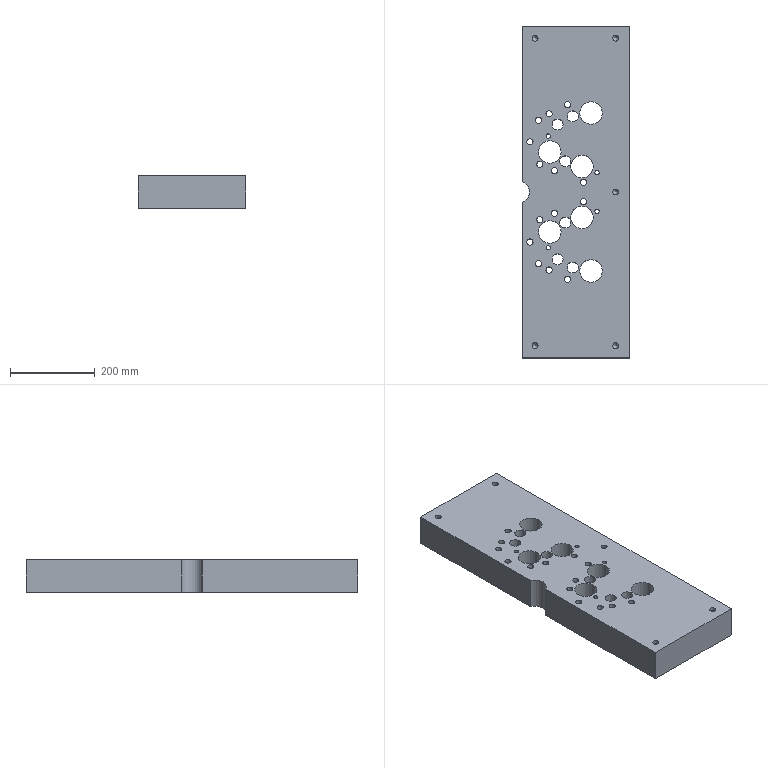Part | NX | features 3 2 | 1 solid | 52 faces | box 253 x 782.437 x 75.5 mm | volume 13452041 mm3 | cylinder 38 | plane 7 | cone 7 | commonest cylinder face diameters 14.5 x14 14.1 x7 53 x7 26 x6 10 x4
STEP:
#1=CARTESIAN_POINT('',(2107.05,-362.5,256.5));
#2=VERTEX_POINT('',#1);
#3=CARTESIAN_POINT('',(2100.,-362.5,256.5));
#4=DIRECTION('',(0.,0.,-1.));
#5=DIRECTION('',(1.,0.,0.));
#6=AXIS2_PLACEMENT_3D('',#3,#4,#5);
#7=CIRCLE('',#6,7.05);
#8=EDGE_CURVE('',#2,#2,#7,.T.);
#9=ORIENTED_EDGE('',*,*,#8,.T.);
#10=EDGE_LOOP('',(#9));
#11=FACE_BOUND('',#10,.T.);
#12=CARTESIAN_POINT('',(1917.05,362.5,256.5));
#13=VERTEX_POINT('',#12);
#14=CARTESIAN_POINT('',(1910.,362.5,256.5));
#15=DIRECTION('',(0.,0.,-1.));
#16=DIRECTION('',(1.,0.,0.));
#17=AXIS2_PLACEMENT_3D('',#14,#15,#16);
#18=CIRCLE('',#17,7.05);
#19=EDGE_CURVE('',#13,#13,#18,.T.);
#20=ORIENTED_EDGE('',*,*,#19,.T.);
#21=EDGE_LOOP('',(#20));
#22=FACE_BOUND('',#21,.T.);
#23=CARTESIAN_POINT('',(2031.25,23.,256.5));
#24=VERTEX_POINT('',#23);
#25=CARTESIAN_POINT('',(2024.,23.,256.5));
#26=DIRECTION('',(0.,0.,-1.));
#27=DIRECTION('',(1.,0.,0.));
#28=AXIS2_PLACEMENT_3D('',#25,#26,#27);
#29=CIRCLE('',#28,7.25);
#30=EDGE_CURVE('',#24,#24,#29,.T.);
#31=ORIENTED_EDGE('',*,*,#30,.T.);
#32=EDGE_LOOP('',(#31));
#33=FACE_BOUND('',#32,.T.);
#34=CARTESIAN_POINT('',(1963.25,50.,256.5));
#35=VERTEX_POINT('',#34);
#36=CARTESIAN_POINT('',(1956.,50.,256.5));
#37=DIRECTION('',(0.,0.,1.));
#38=DIRECTION('',(1.,0.,0.));
#39=AXIS2_PLACEMENT_3D('',#36,#37,#38);
#40=CIRCLE('',#39,7.25);
#41=EDGE_CURVE('',#35,#35,#40,.T.);
#42=ORIENTED_EDGE('',*,*,#41,.F.);
#43=EDGE_LOOP('',(#42));
#44=FACE_BOUND('',#43,.T.);
#45=CARTESIAN_POINT('',(1928.25,65.,256.5));
#46=VERTEX_POINT('',#45);
#47=CARTESIAN_POINT('',(1921.,65.,256.5));
#48=DIRECTION('',(0.,0.,-1.));
#49=DIRECTION('',(1.,0.,0.));
#50=AXIS2_PLACEMENT_3D('',#47,#48,#49);
#51=CIRCLE('',#50,7.25);
#52=EDGE_CURVE('',#46,#46,#51,.T.);
#53=ORIENTED_EDGE('',*,*,#52,.T.);
#54=EDGE_LOOP('',(#53));
#55=FACE_BOUND('',#54,.T.);
#56=CARTESIAN_POINT('',(1905.25,118.,256.5));
#57=VERTEX_POINT('',#56);
#58=CARTESIAN_POINT('',(1898.,118.,256.5));
#59=DIRECTION('',(0.,0.,-1.));
#60=DIRECTION('',(1.,0.,0.));
#61=AXIS2_PLACEMENT_3D('',#58,#59,#60);
#62=CIRCLE('',#61,7.25);
#63=EDGE_CURVE('',#57,#57,#62,.T.);
#64=ORIENTED_EDGE('',*,*,#63,.T.);
#65=EDGE_LOOP('',(#64));
#66=FACE_BOUND('',#65,.T.);
#67=CARTESIAN_POINT('',(1925.25,-169.,256.5));
#68=VERTEX_POINT('',#67);
#69=CARTESIAN_POINT('',(1918.,-169.,256.5));
#70=DIRECTION('',(0.,0.,-1.));
#71=DIRECTION('',(1.,0.,0.));
#72=AXIS2_PLACEMENT_3D('',#69,#70,#71);
#73=CIRCLE('',#72,7.25);
#74=EDGE_CURVE('',#68,#68,#73,.T.);
#75=ORIENTED_EDGE('',*,*,#74,.T.);
#76=EDGE_LOOP('',(#75));
#77=FACE_BOUND('',#76,.T.);
#78=CARTESIAN_POINT('',(1950.25,-184.,256.5));
#79=VERTEX_POINT('',#78);
#80=CARTESIAN_POINT('',(1943.,-184.,256.5));
#81=DIRECTION('',(0.,0.,-1.));
#82=DIRECTION('',(1.,0.,0.));
#83=AXIS2_PLACEMENT_3D('',#80,#81,#82);
#84=CIRCLE('',#83,7.25);
#85=EDGE_CURVE('',#79,#79,#84,.T.);
#86=ORIENTED_EDGE('',*,*,#85,.T.);
#87=EDGE_LOOP('',(#86));
#88=FACE_BOUND('',#87,.T.);
#89=CARTESIAN_POINT('',(1993.25,-206.,256.5));
#90=VERTEX_POINT('',#89);
#91=CARTESIAN_POINT('',(1986.,-206.,256.5));
#92=DIRECTION('',(0.,0.,1.));
#93=DIRECTION('',(1.,0.,0.));
#94=AXIS2_PLACEMENT_3D('',#91,#92,#93);
#95=CIRCLE('',#94,7.25);
#96=EDGE_CURVE('',#90,#90,#95,.T.);
#97=ORIENTED_EDGE('',*,*,#96,.F.);
#98=EDGE_LOOP('',(#97));
#99=FACE_BOUND('',#98,.T.);
#100=CARTESIAN_POINT('',(2012.,-178.,256.5));
#101=VERTEX_POINT('',#100);
#102=CARTESIAN_POINT('',(1999.,-178.,256.5));
#103=DIRECTION('',(0.,0.,-1.));
#104=DIRECTION('',(1.,0.,0.));
#105=AXIS2_PLACEMENT_3D('',#102,#103,#104);
#106=CIRCLE('',#105,13.);
#107=EDGE_CURVE('',#101,#101,#106,.T.);
#108=ORIENTED_EDGE('',*,*,#107,.T.);
#109=EDGE_LOOP('',(#108));
#110=FACE_BOUND('',#109,.T.);
#111=CARTESIAN_POINT('',(1994.,72.,256.5));
#112=VERTEX_POINT('',#111);
#113=CARTESIAN_POINT('',(1981.,72.,256.5));
#114=DIRECTION('',(0.,0.,-1.));
#115=DIRECTION('',(1.,0.,0.));
#116=AXIS2_PLACEMENT_3D('',#113,#114,#115);
#117=CIRCLE('',#116,13.);
#118=EDGE_CURVE('',#112,#112,#117,.T.);
#119=ORIENTED_EDGE('',*,*,#118,.T.);
#120=EDGE_LOOP('',(#119));
#121=FACE_BOUND('',#120,.T.);
#122=CARTESIAN_POINT('',(1994.,-72.,256.5));
#123=VERTEX_POINT('',#122);
#124=CARTESIAN_POINT('',(1981.,-72.,256.5));
#125=DIRECTION('',(0.,0.,-1.));
#126=DIRECTION('',(1.,0.,0.));
#127=AXIS2_PLACEMENT_3D('',#124,#125,#126);
#128=CIRCLE('',#127,13.);
#129=EDGE_CURVE('',#123,#123,#128,.T.);
#130=ORIENTED_EDGE('',*,*,#129,.T.);
#131=EDGE_LOOP('',(#130));
#132=FACE_BOUND('',#131,.T.);
#133=CARTESIAN_POINT('',(1976.,159.,256.5));
#134=VERTEX_POINT('',#133);
#135=CARTESIAN_POINT('',(1963.,159.,256.5));
#136=DIRECTION('',(0.,0.,-1.));
#137=DIRECTION('',(1.,0.,0.));
#138=AXIS2_PLACEMENT_3D('',#135,#136,#137);
#139=CIRCLE('',#138,13.);
#140=EDGE_CURVE('',#134,#134,#139,.T.);
#141=ORIENTED_EDGE('',*,*,#140,.T.);
#142=EDGE_LOOP('',(#141));
#143=FACE_BOUND('',#142,.T.);
#144=CARTESIAN_POINT('',(1976.,-159.,256.5));
#145=VERTEX_POINT('',#144);
#146=CARTESIAN_POINT('',(1963.,-159.,256.5));
#147=DIRECTION('',(0.,0.,-1.));
#148=DIRECTION('',(1.,0.,0.));
#149=AXIS2_PLACEMENT_3D('',#146,#147,#148);
#150=CIRCLE('',#149,13.);
#151=EDGE_CURVE('',#145,#145,#150,.T.);
#152=ORIENTED_EDGE('',*,*,#151,.T.);
#153=EDGE_LOOP('',(#152));
#154=FACE_BOUND('',#153,.T.);
#155=CARTESIAN_POINT('',(1945.861,131.692,256.5));
#156=VERTEX_POINT('',#155);
#157=CARTESIAN_POINT('',(1940.861,131.692,256.5));
#158=DIRECTION('',(0.,0.,-1.));
#159=DIRECTION('',(1.,0.,0.));
#160=AXIS2_PLACEMENT_3D('',#157,#158,#159);
#161=CIRCLE('',#160,5.);
#162=EDGE_CURVE('',#156,#156,#161,.T.);
#163=ORIENTED_EDGE('',*,*,#162,.T.);
#164=EDGE_LOOP('',(#163));
#165=FACE_BOUND('',#164,.T.);
#166=CARTESIAN_POINT('',(2012.,178.,256.5));
#167=VERTEX_POINT('',#166);
#168=CARTESIAN_POINT('',(1999.,178.,256.5));
#169=DIRECTION('',(0.,0.,-1.));
#170=DIRECTION('',(1.,0.,0.));
#171=AXIS2_PLACEMENT_3D('',#168,#169,#170);
#172=CIRCLE('',#171,13.);
#173=EDGE_CURVE('',#167,#167,#172,.T.);
#174=ORIENTED_EDGE('',*,*,#173,.T.);
#175=EDGE_LOOP('',(#174));
#176=FACE_BOUND('',#175,.T.);
#177=CARTESIAN_POINT('',(2060.861,-45.692,256.5));
#178=VERTEX_POINT('',#177);
#179=CARTESIAN_POINT('',(2055.861,-45.692,256.5));
#180=DIRECTION('',(0.,0.,-1.));
#181=DIRECTION('',(1.,0.,0.));
#182=AXIS2_PLACEMENT_3D('',#179,#180,#181);
#183=CIRCLE('',#182,5.);
#184=EDGE_CURVE('',#178,#178,#183,.T.);
#185=ORIENTED_EDGE('',*,*,#184,.T.);
#186=EDGE_LOOP('',(#185));
#187=FACE_BOUND('',#186,.T.);
#188=CARTESIAN_POINT('',(2060.861,45.692,256.5));
#189=VERTEX_POINT('',#188);
#190=CARTESIAN_POINT('',(2055.861,45.692,256.5));
#191=DIRECTION('',(0.,0.,-1.));
#192=DIRECTION('',(1.,0.,0.));
#193=AXIS2_PLACEMENT_3D('',#190,#191,#192);
#194=CIRCLE('',#193,5.);
#195=EDGE_CURVE('',#189,#189,#194,.T.);
#196=ORIENTED_EDGE('',*,*,#195,.T.);
#197=EDGE_LOOP('',(#196));
#198=FACE_BOUND('',#197,.T.);
#199=CARTESIAN_POINT('',(2047.195,60.048,256.5));
#200=VERTEX_POINT('',#199);
#201=CARTESIAN_POINT('',(2020.695,60.048,256.5));
#202=DIRECTION('',(0.,0.,-1.));
#203=DIRECTION('',(1.,0.,0.));
#204=AXIS2_PLACEMENT_3D('',#201,#202,#203);
#205=CIRCLE('',#204,26.5);
#206=EDGE_CURVE('',#200,#200,#205,.T.);
#207=ORIENTED_EDGE('',*,*,#206,.T.);
#208=EDGE_LOOP('',(#207));
#209=FACE_BOUND('',#208,.T.);
#210=CARTESIAN_POINT('',(2047.195,-60.048,256.5));
#211=VERTEX_POINT('',#210);
#212=CARTESIAN_POINT('',(2020.695,-60.048,256.5));
#213=DIRECTION('',(0.,0.,-1.));
#214=DIRECTION('',(1.,0.,0.));
#215=AXIS2_PLACEMENT_3D('',#212,#213,#214);
#216=CIRCLE('',#215,26.5);
#217=EDGE_CURVE('',#211,#211,#216,.T.);
#218=ORIENTED_EDGE('',*,*,#217,.T.);
#219=EDGE_LOOP('',(#218));
#220=FACE_BOUND('',#219,.T.);
#221=CARTESIAN_POINT('',(2068.5,-186.,256.5));
#222=VERTEX_POINT('',#221);
#223=CARTESIAN_POINT('',(2042.,-186.,256.5));
#224=DIRECTION('',(0.,0.,-1.));
#225=DIRECTION('',(1.,0.,0.));
#226=AXIS2_PLACEMENT_3D('',#223,#224,#225);
#227=CIRCLE('',#226,26.5);
#228=EDGE_CURVE('',#222,#222,#227,.T.);
#229=ORIENTED_EDGE('',*,*,#228,.T.);
#230=EDGE_LOOP('',(#229));
#231=FACE_BOUND('',#230,.T.);
#232=CARTESIAN_POINT('',(1971.5,94.,256.5));
#233=VERTEX_POINT('',#232);
#234=CARTESIAN_POINT('',(1945.,94.,256.5));
#235=DIRECTION('',(0.,0.,1.));
#236=DIRECTION('',(1.,0.,0.));
#237=AXIS2_PLACEMENT_3D('',#234,#235,#236);
#238=CIRCLE('',#237,26.5);
#239=EDGE_CURVE('',#233,#233,#238,.T.);
#240=ORIENTED_EDGE('',*,*,#239,.F.);
#241=EDGE_LOOP('',(#240));
#242=FACE_BOUND('',#241,.T.);
#243=CARTESIAN_POINT('',(1880.,-24.541,256.5));
#244=VERTEX_POINT('',#243);
#245=CARTESIAN_POINT('',(1880.,24.541,256.5));
#246=VERTEX_POINT('',#245);
#247=CARTESIAN_POINT('',(1870.,0.,256.5));
#248=DIRECTION('',(0.,0.,1.));
#249=DIRECTION('',(1.,0.,0.));
#250=AXIS2_PLACEMENT_3D('',#247,#248,#249);
#251=CIRCLE('',#250,26.5);
#252=EDGE_CURVE('',#244,#246,#251,.T.);
#253=ORIENTED_EDGE('',*,*,#252,.F.);
#254=CARTESIAN_POINT('',(1880.,-391.218,256.5));
#255=VERTEX_POINT('',#254);
#256=CARTESIAN_POINT('',(1880.,193.,256.5));
#257=DIRECTION('',(0.,1.,0.));
#258=VECTOR('',#257,1000.);
#259=LINE('',#256,#258);
#260=EDGE_CURVE('',#255,#244,#259,.T.);
#261=ORIENTED_EDGE('',*,*,#260,.F.);
#262=CARTESIAN_POINT('',(2133.,-391.218,256.5));
#263=VERTEX_POINT('',#262);
#264=CARTESIAN_POINT('',(4065.,-391.218,256.5));
#265=DIRECTION('',(1.,0.,0.));
#266=VECTOR('',#265,1000.);
#267=LINE('',#264,#266);
#268=EDGE_CURVE('',#255,#263,#267,.T.);
#269=ORIENTED_EDGE('',*,*,#268,.T.);
#270=CARTESIAN_POINT('',(2133.,391.218,256.5));
#271=VERTEX_POINT('',#270);
#272=CARTESIAN_POINT('',(2133.,193.,256.5));
#273=DIRECTION('',(0.,-1.,0.));
#274=VECTOR('',#273,1000.);
#275=LINE('',#272,#274);
#276=EDGE_CURVE('',#271,#263,#275,.T.);
#277=ORIENTED_EDGE('',*,*,#276,.F.);
#278=CARTESIAN_POINT('',(1880.,391.218,256.5));
#279=VERTEX_POINT('',#278);
#280=CARTESIAN_POINT('',(4065.,391.218,256.5));
#281=DIRECTION('',(1.,0.,0.));
#282=VECTOR('',#281,1000.);
#283=LINE('',#280,#282);
#284=EDGE_CURVE('',#279,#271,#283,.T.);
#285=ORIENTED_EDGE('',*,*,#284,.F.);
#286=CARTESIAN_POINT('',(1880.,193.,256.5));
#287=DIRECTION('',(0.,1.,0.));
#288=VECTOR('',#287,1000.);
#289=LINE('',#286,#288);
#290=EDGE_CURVE('',#246,#279,#289,.T.);
#291=ORIENTED_EDGE('',*,*,#290,.F.);
#292=EDGE_LOOP('',(#253,#261,#269,#277,#285,#291));
#293=FACE_BOUND('',#292,.T.);
#294=CARTESIAN_POINT('',(1971.5,-94.,256.5));
#295=VERTEX_POINT('',#294);
#296=CARTESIAN_POINT('',(1945.,-94.,256.5));
#297=DIRECTION('',(0.,0.,-1.));
#298=DIRECTION('',(1.,0.,0.));
#299=AXIS2_PLACEMENT_3D('',#296,#297,#298);
#300=CIRCLE('',#299,26.5);
#301=EDGE_CURVE('',#295,#295,#300,.T.);
#302=ORIENTED_EDGE('',*,*,#301,.T.);
#303=EDGE_LOOP('',(#302));
#304=FACE_BOUND('',#303,.T.);
#305=CARTESIAN_POINT('',(2068.5,186.,256.5));
#306=VERTEX_POINT('',#305);
#307=CARTESIAN_POINT('',(2042.,186.,256.5));
#308=DIRECTION('',(0.,0.,1.));
#309=DIRECTION('',(1.,0.,0.));
#310=AXIS2_PLACEMENT_3D('',#307,#308,#309);
#311=CIRCLE('',#310,26.5);
#312=EDGE_CURVE('',#306,#306,#311,.T.);
#313=ORIENTED_EDGE('',*,*,#312,.F.);
#314=EDGE_LOOP('',(#313));
#315=FACE_BOUND('',#314,.T.);
#316=CARTESIAN_POINT('',(1945.861,-131.692,256.5));
#317=VERTEX_POINT('',#316);
#318=CARTESIAN_POINT('',(1940.861,-131.692,256.5));
#319=DIRECTION('',(0.,0.,-1.));
#320=DIRECTION('',(1.,0.,0.));
#321=AXIS2_PLACEMENT_3D('',#318,#319,#320);
#322=CIRCLE('',#321,5.);
#323=EDGE_CURVE('',#317,#317,#322,.T.);
#324=ORIENTED_EDGE('',*,*,#323,.T.);
#325=EDGE_LOOP('',(#324));
#326=FACE_BOUND('',#325,.T.);
#327=CARTESIAN_POINT('',(2031.25,-23.,256.5));
#328=VERTEX_POINT('',#327);
#329=CARTESIAN_POINT('',(2024.,-23.,256.5));
#330=DIRECTION('',(0.,0.,-1.));
#331=DIRECTION('',(1.,0.,0.));
#332=AXIS2_PLACEMENT_3D('',#329,#330,#331);
#333=CIRCLE('',#332,7.25);
#334=EDGE_CURVE('',#328,#328,#333,.T.);
#335=ORIENTED_EDGE('',*,*,#334,.T.);
#336=EDGE_LOOP('',(#335));
#337=FACE_BOUND('',#336,.T.);
#338=CARTESIAN_POINT('',(1963.25,-50.,256.5));
#339=VERTEX_POINT('',#338);
#340=CARTESIAN_POINT('',(1956.,-50.,256.5));
#341=DIRECTION('',(0.,0.,-1.));
#342=DIRECTION('',(1.,0.,0.));
#343=AXIS2_PLACEMENT_3D('',#340,#341,#342);
#344=CIRCLE('',#343,7.25);
#345=EDGE_CURVE('',#339,#339,#344,.T.);
#346=ORIENTED_EDGE('',*,*,#345,.T.);
#347=EDGE_LOOP('',(#346));
#348=FACE_BOUND('',#347,.T.);
#349=CARTESIAN_POINT('',(1928.25,-65.,256.5));
#350=VERTEX_POINT('',#349);
#351=CARTESIAN_POINT('',(1921.,-65.,256.5));
#352=DIRECTION('',(0.,0.,1.));
#353=DIRECTION('',(1.,0.,0.));
#354=AXIS2_PLACEMENT_3D('',#351,#352,#353);
#355=CIRCLE('',#354,7.25);
#356=EDGE_CURVE('',#350,#350,#355,.T.);
#357=ORIENTED_EDGE('',*,*,#356,.F.);
#358=EDGE_LOOP('',(#357));
#359=FACE_BOUND('',#358,.T.);
#360=CARTESIAN_POINT('',(1905.25,-118.,256.5));
#361=VERTEX_POINT('',#360);
#362=CARTESIAN_POINT('',(1898.,-118.,256.5));
#363=DIRECTION('',(0.,0.,-1.));
#364=DIRECTION('',(1.,0.,0.));
#365=AXIS2_PLACEMENT_3D('',#362,#363,#364);
#366=CIRCLE('',#365,7.25);
#367=EDGE_CURVE('',#361,#361,#366,.T.);
#368=ORIENTED_EDGE('',*,*,#367,.T.);
#369=EDGE_LOOP('',(#368));
#370=FACE_BOUND('',#369,.T.);
#371=CARTESIAN_POINT('',(1925.25,169.,256.5));
#372=VERTEX_POINT('',#371);
#373=CARTESIAN_POINT('',(1918.,169.,256.5));
#374=DIRECTION('',(0.,0.,-1.));
#375=DIRECTION('',(1.,0.,0.));
#376=AXIS2_PLACEMENT_3D('',#373,#374,#375);
#377=CIRCLE('',#376,7.25);
#378=EDGE_CURVE('',#372,#372,#377,.T.);
#379=ORIENTED_EDGE('',*,*,#378,.T.);
#380=EDGE_LOOP('',(#379));
#381=FACE_BOUND('',#380,.T.);
#382=CARTESIAN_POINT('',(1950.25,184.,256.5));
#383=VERTEX_POINT('',#382);
#384=CARTESIAN_POINT('',(1943.,184.,256.5));
#385=DIRECTION('',(0.,0.,-1.));
#386=DIRECTION('',(1.,0.,0.));
#387=AXIS2_PLACEMENT_3D('',#384,#385,#386);
#388=CIRCLE('',#387,7.25);
#389=EDGE_CURVE('',#383,#383,#388,.T.);
#390=ORIENTED_EDGE('',*,*,#389,.T.);
#391=EDGE_LOOP('',(#390));
#392=FACE_BOUND('',#391,.T.);
#393=CARTESIAN_POINT('',(1993.25,206.,256.5));
#394=VERTEX_POINT('',#393);
#395=CARTESIAN_POINT('',(1986.,206.,256.5));
#396=DIRECTION('',(0.,0.,-1.));
#397=DIRECTION('',(1.,0.,0.));
#398=AXIS2_PLACEMENT_3D('',#395,#396,#397);
#399=CIRCLE('',#398,7.25);
#400=EDGE_CURVE('',#394,#394,#399,.T.);
#401=ORIENTED_EDGE('',*,*,#400,.T.);
#402=EDGE_LOOP('',(#401));
#403=FACE_BOUND('',#402,.T.);
#404=CARTESIAN_POINT('',(1917.05,-362.5,256.5));
#405=VERTEX_POINT('',#404);
#406=CARTESIAN_POINT('',(1910.,-362.5,256.5));
#407=DIRECTION('',(0.,0.,-1.));
#408=DIRECTION('',(1.,0.,0.));
#409=AXIS2_PLACEMENT_3D('',#406,#407,#408);
#410=CIRCLE('',#409,7.05);
#411=EDGE_CURVE('',#405,#405,#410,.T.);
#412=ORIENTED_EDGE('',*,*,#411,.T.);
#413=EDGE_LOOP('',(#412));
#414=FACE_BOUND('',#413,.T.);
#415=CARTESIAN_POINT('',(2107.05,362.5,256.5));
#416=VERTEX_POINT('',#415);
#417=CARTESIAN_POINT('',(2100.,362.5,256.5));
#418=DIRECTION('',(0.,0.,-1.));
#419=DIRECTION('',(1.,0.,0.));
#420=AXIS2_PLACEMENT_3D('',#417,#418,#419);
#421=CIRCLE('',#420,7.05);
#422=EDGE_CURVE('',#416,#416,#421,.T.);
#423=ORIENTED_EDGE('',*,*,#422,.T.);
#424=EDGE_LOOP('',(#423));
#425=FACE_BOUND('',#424,.T.);
#426=CARTESIAN_POINT('',(2107.05,0.,256.5));
#427=VERTEX_POINT('',#426);
#428=CARTESIAN_POINT('',(2100.,0.,256.5));
#429=DIRECTION('',(0.,0.,-1.));
#430=DIRECTION('',(1.,0.,0.));
#431=AXIS2_PLACEMENT_3D('',#428,#429,#430);
#432=CIRCLE('',#431,7.05);
#433=EDGE_CURVE('',#427,#427,#432,.T.);
#434=ORIENTED_EDGE('',*,*,#433,.T.);
#435=EDGE_LOOP('',(#434));
#436=FACE_BOUND('',#435,.T.);
#437=CARTESIAN_POINT('',(4065.,0.,256.5));
#438=DIRECTION('',(0.,0.,1.));
#439=DIRECTION('',(-1.,0.,0.));
#440=AXIS2_PLACEMENT_3D('',#437,#438,#439);
#441=PLANE('',#440);
#442=ADVANCED_FACE('',(#11,#22,#33,#44,#55,#66,#77,#88,#99,#110,#121,#132,#143,#154,#165,#176,#187,#198,#209,#220,#231,#242,#293,#304,#315,#326,#337,#348,#359,#370,#381,#392,#403,#414,#425,#436),#441,.T.);
#443=CARTESIAN_POINT('',(1935.861,131.692,181.));
#444=VERTEX_POINT('',#443);
#445=CARTESIAN_POINT('',(1940.861,131.692,181.));
#446=DIRECTION('',(0.,0.,-1.));
#447=DIRECTION('',(-1.,0.,0.));
#448=AXIS2_PLACEMENT_3D('',#445,#446,#447);
#449=CIRCLE('',#448,5.);
#450=EDGE_CURVE('',#444,#444,#449,.T.);
#451=ORIENTED_EDGE('',*,*,#450,.F.);
#452=EDGE_LOOP('',(#451));
#453=FACE_BOUND('',#452,.T.);
#454=CARTESIAN_POINT('',(2050.861,45.692,181.));
#455=VERTEX_POINT('',#454);
#456=CARTESIAN_POINT('',(2055.861,45.692,181.));
#457=DIRECTION('',(0.,0.,-1.));
#458=DIRECTION('',(-1.,0.,0.));
#459=AXIS2_PLACEMENT_3D('',#456,#457,#458);
#460=CIRCLE('',#459,5.);
#461=EDGE_CURVE('',#455,#455,#460,.T.);
#462=ORIENTED_EDGE('',*,*,#461,.F.);
#463=EDGE_LOOP('',(#462));
#464=FACE_BOUND('',#463,.T.);
#465=CARTESIAN_POINT('',(2050.861,-45.692,181.));
#466=VERTEX_POINT('',#465);
#467=CARTESIAN_POINT('',(2055.861,-45.692,181.));
#468=DIRECTION('',(0.,0.,-1.));
#469=DIRECTION('',(-1.,0.,0.));
#470=AXIS2_PLACEMENT_3D('',#467,#468,#469);
#471=CIRCLE('',#470,5.);
#472=EDGE_CURVE('',#466,#466,#471,.T.);
#473=ORIENTED_EDGE('',*,*,#472,.F.);
#474=EDGE_LOOP('',(#473));
#475=FACE_BOUND('',#474,.T.);
#476=CARTESIAN_POINT('',(1935.861,-131.692,181.));
#477=VERTEX_POINT('',#476);
#478=CARTESIAN_POINT('',(1940.861,-131.692,181.));
#479=DIRECTION('',(0.,0.,-1.));
#480=DIRECTION('',(-1.,0.,0.));
#481=AXIS2_PLACEMENT_3D('',#478,#479,#480);
#482=CIRCLE('',#481,5.);
#483=EDGE_CURVE('',#477,#477,#482,.T.);
#484=ORIENTED_EDGE('',*,*,#483,.F.);
#485=EDGE_LOOP('',(#484));
#486=FACE_BOUND('',#485,.T.);
#487=CARTESIAN_POINT('',(1917.05,-362.5,181.));
#488=VERTEX_POINT('',#487);
#489=CARTESIAN_POINT('',(1910.,-362.5,181.));
#490=DIRECTION('',(0.,0.,1.));
#491=DIRECTION('',(1.,0.,0.));
#492=AXIS2_PLACEMENT_3D('',#489,#490,#491);
#493=CIRCLE('',#492,7.05);
#494=EDGE_CURVE('',#488,#488,#493,.T.);
#495=ORIENTED_EDGE('',*,*,#494,.T.);
#496=EDGE_LOOP('',(#495));
#497=FACE_BOUND('',#496,.T.);
#498=CARTESIAN_POINT('',(1978.75,206.,181.));
#499=VERTEX_POINT('',#498);
#500=CARTESIAN_POINT('',(1986.,206.,181.));
#501=DIRECTION('',(0.,0.,-1.));
#502=DIRECTION('',(-1.,0.,0.));
#503=AXIS2_PLACEMENT_3D('',#500,#501,#502);
#504=CIRCLE('',#503,7.25);
#505=EDGE_CURVE('',#499,#499,#504,.T.);
#506=ORIENTED_EDGE('',*,*,#505,.F.);
#507=EDGE_LOOP('',(#506));
#508=FACE_BOUND('',#507,.T.);
#509=CARTESIAN_POINT('',(1935.75,184.,181.));
#510=VERTEX_POINT('',#509);
#511=CARTESIAN_POINT('',(1943.,184.,181.));
#512=DIRECTION('',(0.,0.,-1.));
#513=DIRECTION('',(-1.,0.,0.));
#514=AXIS2_PLACEMENT_3D('',#511,#512,#513);
#515=CIRCLE('',#514,7.25);
#516=EDGE_CURVE('',#510,#510,#515,.T.);
#517=ORIENTED_EDGE('',*,*,#516,.F.);
#518=EDGE_LOOP('',(#517));
#519=FACE_BOUND('',#518,.T.);
#520=CARTESIAN_POINT('',(1910.75,169.,181.));
#521=VERTEX_POINT('',#520);
#522=CARTESIAN_POINT('',(1918.,169.,181.));
#523=DIRECTION('',(0.,0.,1.));
#524=DIRECTION('',(-1.,0.,0.));
#525=AXIS2_PLACEMENT_3D('',#522,#523,#524);
#526=CIRCLE('',#525,7.25);
#527=EDGE_CURVE('',#521,#521,#526,.T.);
#528=ORIENTED_EDGE('',*,*,#527,.T.);
#529=EDGE_LOOP('',(#528));
#530=FACE_BOUND('',#529,.T.);
#531=CARTESIAN_POINT('',(1890.75,-118.,181.));
#532=VERTEX_POINT('',#531);
#533=CARTESIAN_POINT('',(1898.,-118.,181.));
#534=DIRECTION('',(0.,0.,1.));
#535=DIRECTION('',(-1.,0.,0.));
#536=AXIS2_PLACEMENT_3D('',#533,#534,#535);
#537=CIRCLE('',#536,7.25);
#538=EDGE_CURVE('',#532,#532,#537,.T.);
#539=ORIENTED_EDGE('',*,*,#538,.T.);
#540=EDGE_LOOP('',(#539));
#541=FACE_BOUND('',#540,.T.);
#542=CARTESIAN_POINT('',(1913.75,-65.,181.));
#543=VERTEX_POINT('',#542);
#544=CARTESIAN_POINT('',(1921.,-65.,181.));
#545=DIRECTION('',(0.,0.,1.));
#546=DIRECTION('',(-1.,0.,0.));
#547=AXIS2_PLACEMENT_3D('',#544,#545,#546);
#548=CIRCLE('',#547,7.25);
#549=EDGE_CURVE('',#543,#543,#548,.T.);
#550=ORIENTED_EDGE('',*,*,#549,.T.);
#551=EDGE_LOOP('',(#550));
#552=FACE_BOUND('',#551,.T.);
#553=CARTESIAN_POINT('',(1948.75,-50.,181.));
#554=VERTEX_POINT('',#553);
#555=CARTESIAN_POINT('',(1956.,-50.,181.));
#556=DIRECTION('',(0.,0.,-1.));
#557=DIRECTION('',(-1.,0.,0.));
#558=AXIS2_PLACEMENT_3D('',#555,#556,#557);
#559=CIRCLE('',#558,7.25);
#560=EDGE_CURVE('',#554,#554,#559,.T.);
#561=ORIENTED_EDGE('',*,*,#560,.F.);
#562=EDGE_LOOP('',(#561));
#563=FACE_BOUND('',#562,.T.);
#564=CARTESIAN_POINT('',(2016.75,-23.,181.));
#565=VERTEX_POINT('',#564);
#566=CARTESIAN_POINT('',(2024.,-23.,181.));
#567=DIRECTION('',(0.,0.,1.));
#568=DIRECTION('',(-1.,0.,0.));
#569=AXIS2_PLACEMENT_3D('',#566,#567,#568);
#570=CIRCLE('',#569,7.25);
#571=EDGE_CURVE('',#565,#565,#570,.T.);
#572=ORIENTED_EDGE('',*,*,#571,.T.);
#573=EDGE_LOOP('',(#572));
#574=FACE_BOUND('',#573,.T.);
#575=CARTESIAN_POINT('',(2015.5,186.,181.));
#576=VERTEX_POINT('',#575);
#577=CARTESIAN_POINT('',(2042.,186.,181.));
#578=DIRECTION('',(0.,0.,1.));
#579=DIRECTION('',(-1.,0.,0.));
#580=AXIS2_PLACEMENT_3D('',#577,#578,#579);
#581=CIRCLE('',#580,26.5);
#582=EDGE_CURVE('',#576,#576,#581,.T.);
#583=ORIENTED_EDGE('',*,*,#582,.T.);
#584=EDGE_LOOP('',(#583));
#585=FACE_BOUND('',#584,.T.);
#586=CARTESIAN_POINT('',(1918.5,-94.,181.));
#587=VERTEX_POINT('',#586);
#588=CARTESIAN_POINT('',(1945.,-94.,181.));
#589=DIRECTION('',(0.,0.,-1.));
#590=DIRECTION('',(-1.,0.,0.));
#591=AXIS2_PLACEMENT_3D('',#588,#589,#590);
#592=CIRCLE('',#591,26.5);
#593=EDGE_CURVE('',#587,#587,#592,.T.);
#594=ORIENTED_EDGE('',*,*,#593,.F.);
#595=EDGE_LOOP('',(#594));
#596=FACE_BOUND('',#595,.T.);
#597=CARTESIAN_POINT('',(1880.,-24.541,181.));
#598=VERTEX_POINT('',#597);
#599=CARTESIAN_POINT('',(1880.,24.541,181.));
#600=VERTEX_POINT('',#599);
#601=CARTESIAN_POINT('',(1870.,0.,181.));
#602=DIRECTION('',(0.,0.,1.));
#603=DIRECTION('',(-1.,0.,0.));
#604=AXIS2_PLACEMENT_3D('',#601,#602,#603);
#605=CIRCLE('',#604,26.5);
#606=EDGE_CURVE('',#598,#600,#605,.T.);
#607=ORIENTED_EDGE('',*,*,#606,.T.);
#608=CARTESIAN_POINT('',(1880.,391.218,181.));
#609=VERTEX_POINT('',#608);
#610=CARTESIAN_POINT('',(1880.,193.,181.));
#611=DIRECTION('',(0.,-1.,0.));
#612=VECTOR('',#611,1000.);
#613=LINE('',#610,#612);
#614=EDGE_CURVE('',#609,#600,#613,.T.);
#615=ORIENTED_EDGE('',*,*,#614,.F.);
#616=CARTESIAN_POINT('',(2133.,391.218,181.));
#617=VERTEX_POINT('',#616);
#618=CARTESIAN_POINT('',(3295.,391.218,181.));
#619=DIRECTION('',(-1.,0.,0.));
#620=VECTOR('',#619,1000.);
#621=LINE('',#618,#620);
#622=EDGE_CURVE('',#617,#609,#621,.T.);
#623=ORIENTED_EDGE('',*,*,#622,.F.);
#624=CARTESIAN_POINT('',(2133.,-391.218,181.));
#625=VERTEX_POINT('',#624);
#626=CARTESIAN_POINT('',(2133.,193.,181.));
#627=DIRECTION('',(0.,1.,0.));
#628=VECTOR('',#627,1000.);
#629=LINE('',#626,#628);
#630=EDGE_CURVE('',#625,#617,#629,.T.);
#631=ORIENTED_EDGE('',*,*,#630,.F.);
#632=CARTESIAN_POINT('',(1880.,-391.218,181.));
#633=VERTEX_POINT('',#632);
#634=CARTESIAN_POINT('',(3295.,-391.218,181.));
#635=DIRECTION('',(-1.,0.,0.));
#636=VECTOR('',#635,1000.);
#637=LINE('',#634,#636);
#638=EDGE_CURVE('',#625,#633,#637,.T.);
#639=ORIENTED_EDGE('',*,*,#638,.T.);
#640=CARTESIAN_POINT('',(1880.,193.,181.));
#641=DIRECTION('',(0.,-1.,0.));
#642=VECTOR('',#641,1000.);
#643=LINE('',#640,#642);
#644=EDGE_CURVE('',#598,#633,#643,.T.);
#645=ORIENTED_EDGE('',*,*,#644,.F.);
#646=EDGE_LOOP('',(#607,#615,#623,#631,#639,#645));
#647=FACE_BOUND('',#646,.T.);
#648=CARTESIAN_POINT('',(1918.5,94.,181.));
#649=VERTEX_POINT('',#648);
#650=CARTESIAN_POINT('',(1945.,94.,181.));
#651=DIRECTION('',(0.,0.,1.));
#652=DIRECTION('',(-1.,0.,0.));
#653=AXIS2_PLACEMENT_3D('',#650,#651,#652);
#654=CIRCLE('',#653,26.5);
#655=EDGE_CURVE('',#649,#649,#654,.T.);
#656=ORIENTED_EDGE('',*,*,#655,.T.);
#657=EDGE_LOOP('',(#656));
#658=FACE_BOUND('',#657,.T.);
#659=CARTESIAN_POINT('',(2015.5,-186.,181.));
#660=VERTEX_POINT('',#659);
#661=CARTESIAN_POINT('',(2042.,-186.,181.));
#662=DIRECTION('',(0.,0.,-1.));
#663=DIRECTION('',(-1.,0.,0.));
#664=AXIS2_PLACEMENT_3D('',#661,#662,#663);
#665=CIRCLE('',#664,26.5);
#666=EDGE_CURVE('',#660,#660,#665,.T.);
#667=ORIENTED_EDGE('',*,*,#666,.F.);
#668=EDGE_LOOP('',(#667));
#669=FACE_BOUND('',#668,.T.);
#670=CARTESIAN_POINT('',(1994.195,-60.048,181.));
#671=VERTEX_POINT('',#670);
#672=CARTESIAN_POINT('',(2020.695,-60.048,181.));
#673=DIRECTION('',(0.,0.,-1.));
#674=DIRECTION('',(-1.,0.,0.));
#675=AXIS2_PLACEMENT_3D('',#672,#673,#674);
#676=CIRCLE('',#675,26.5);
#677=EDGE_CURVE('',#671,#671,#676,.T.);
#678=ORIENTED_EDGE('',*,*,#677,.F.);
#679=EDGE_LOOP('',(#678));
#680=FACE_BOUND('',#679,.T.);
#681=CARTESIAN_POINT('',(1994.195,60.048,181.));
#682=VERTEX_POINT('',#681);
#683=CARTESIAN_POINT('',(2020.695,60.048,181.));
#684=DIRECTION('',(0.,0.,-1.));
#685=DIRECTION('',(-1.,0.,0.));
#686=AXIS2_PLACEMENT_3D('',#683,#684,#685);
#687=CIRCLE('',#686,26.5);
#688=EDGE_CURVE('',#682,#682,#687,.T.);
#689=ORIENTED_EDGE('',*,*,#688,.F.);
#690=EDGE_LOOP('',(#689));
#691=FACE_BOUND('',#690,.T.);
#692=CARTESIAN_POINT('',(1986.,178.,181.));
#693=VERTEX_POINT('',#692);
#694=CARTESIAN_POINT('',(1999.,178.,181.));
#695=DIRECTION('',(0.,0.,1.));
#696=DIRECTION('',(-1.,0.,0.));
#697=AXIS2_PLACEMENT_3D('',#694,#695,#696);
#698=CIRCLE('',#697,13.);
#699=EDGE_CURVE('',#693,#693,#698,.T.);
#700=ORIENTED_EDGE('',*,*,#699,.T.);
#701=EDGE_LOOP('',(#700));
#702=FACE_BOUND('',#701,.T.);
#703=CARTESIAN_POINT('',(1950.,-159.,181.));
#704=VERTEX_POINT('',#703);
#705=CARTESIAN_POINT('',(1963.,-159.,181.));
#706=DIRECTION('',(0.,0.,-1.));
#707=DIRECTION('',(-1.,0.,0.));
#708=AXIS2_PLACEMENT_3D('',#705,#706,#707);
#709=CIRCLE('',#708,13.);
#710=EDGE_CURVE('',#704,#704,#709,.T.);
#711=ORIENTED_EDGE('',*,*,#710,.F.);
#712=EDGE_LOOP('',(#711));
#713=FACE_BOUND('',#712,.T.);
#714=CARTESIAN_POINT('',(1950.,159.,181.));
#715=VERTEX_POINT('',#714);
#716=CARTESIAN_POINT('',(1963.,159.,181.));
#717=DIRECTION('',(0.,0.,1.));
#718=DIRECTION('',(-1.,0.,0.));
#719=AXIS2_PLACEMENT_3D('',#716,#717,#718);
#720=CIRCLE('',#719,13.);
#721=EDGE_CURVE('',#715,#715,#720,.T.);
#722=ORIENTED_EDGE('',*,*,#721,.T.);
#723=EDGE_LOOP('',(#722));
#724=FACE_BOUND('',#723,.T.);
#725=CARTESIAN_POINT('',(1968.,-72.,181.));
#726=VERTEX_POINT('',#725);
#727=CARTESIAN_POINT('',(1981.,-72.,181.));
#728=DIRECTION('',(0.,0.,1.));
#729=DIRECTION('',(-1.,0.,0.));
#730=AXIS2_PLACEMENT_3D('',#727,#728,#729);
#731=CIRCLE('',#730,13.);
#732=EDGE_CURVE('',#726,#726,#731,.T.);
#733=ORIENTED_EDGE('',*,*,#732,.T.);
#734=EDGE_LOOP('',(#733));
#735=FACE_BOUND('',#734,.T.);
#736=CARTESIAN_POINT('',(1968.,72.,181.));
#737=VERTEX_POINT('',#736);
#738=CARTESIAN_POINT('',(1981.,72.,181.));
#739=DIRECTION('',(0.,0.,-1.));
#740=DIRECTION('',(-1.,0.,0.));
#741=AXIS2_PLACEMENT_3D('',#738,#739,#740);
#742=CIRCLE('',#741,13.);
#743=EDGE_CURVE('',#737,#737,#742,.T.);
#744=ORIENTED_EDGE('',*,*,#743,.F.);
#745=EDGE_LOOP('',(#744));
#746=FACE_BOUND('',#745,.T.);
#747=CARTESIAN_POINT('',(1986.,-178.,181.));
#748=VERTEX_POINT('',#747);
#749=CARTESIAN_POINT('',(1999.,-178.,181.));
#750=DIRECTION('',(0.,0.,1.));
#751=DIRECTION('',(-1.,0.,0.));
#752=AXIS2_PLACEMENT_3D('',#749,#750,#751);
#753=CIRCLE('',#752,13.);
#754=EDGE_CURVE('',#748,#748,#753,.T.);
#755=ORIENTED_EDGE('',*,*,#754,.T.);
#756=EDGE_LOOP('',(#755));
#757=FACE_BOUND('',#756,.T.);
#758=CARTESIAN_POINT('',(1978.75,-206.,181.));
#759=VERTEX_POINT('',#758);
#760=CARTESIAN_POINT('',(1986.,-206.,181.));
#761=DIRECTION('',(0.,0.,-1.));
#762=DIRECTION('',(-1.,0.,0.));
#763=AXIS2_PLACEMENT_3D('',#760,#761,#762);
#764=CIRCLE('',#763,7.25);
#765=EDGE_CURVE('',#759,#759,#764,.T.);
#766=ORIENTED_EDGE('',*,*,#765,.F.);
#767=EDGE_LOOP('',(#766));
#768=FACE_BOUND('',#767,.T.);
#769=CARTESIAN_POINT('',(1935.75,-184.,181.));
#770=VERTEX_POINT('',#769);
#771=CARTESIAN_POINT('',(1943.,-184.,181.));
#772=DIRECTION('',(0.,0.,1.));
#773=DIRECTION('',(-1.,0.,0.));
#774=AXIS2_PLACEMENT_3D('',#771,#772,#773);
#775=CIRCLE('',#774,7.25);
#776=EDGE_CURVE('',#770,#770,#775,.T.);
#777=ORIENTED_EDGE('',*,*,#776,.T.);
#778=EDGE_LOOP('',(#777));
#779=FACE_BOUND('',#778,.T.);
#780=CARTESIAN_POINT('',(1910.75,-169.,181.));
#781=VERTEX_POINT('',#780);
#782=CARTESIAN_POINT('',(1918.,-169.,181.));
#783=DIRECTION('',(0.,0.,1.));
#784=DIRECTION('',(-1.,0.,0.));
#785=AXIS2_PLACEMENT_3D('',#782,#783,#784);
#786=CIRCLE('',#785,7.25);
#787=EDGE_CURVE('',#781,#781,#786,.T.);
#788=ORIENTED_EDGE('',*,*,#787,.T.);
#789=EDGE_LOOP('',(#788));
#790=FACE_BOUND('',#789,.T.);
#791=CARTESIAN_POINT('',(1890.75,118.,181.));
#792=VERTEX_POINT('',#791);
#793=CARTESIAN_POINT('',(1898.,118.,181.));
#794=DIRECTION('',(0.,0.,-1.));
#795=DIRECTION('',(-1.,0.,0.));
#796=AXIS2_PLACEMENT_3D('',#793,#794,#795);
#797=CIRCLE('',#796,7.25);
#798=EDGE_CURVE('',#792,#792,#797,.T.);
#799=ORIENTED_EDGE('',*,*,#798,.F.);
#800=EDGE_LOOP('',(#799));
#801=FACE_BOUND('',#800,.T.);
#802=CARTESIAN_POINT('',(1913.75,65.,181.));
#803=VERTEX_POINT('',#802);
#804=CARTESIAN_POINT('',(1921.,65.,181.));
#805=DIRECTION('',(0.,0.,-1.));
#806=DIRECTION('',(-1.,0.,0.));
#807=AXIS2_PLACEMENT_3D('',#804,#805,#806);
#808=CIRCLE('',#807,7.25);
#809=EDGE_CURVE('',#803,#803,#808,.T.);
#810=ORIENTED_EDGE('',*,*,#809,.F.);
#811=EDGE_LOOP('',(#810));
#812=FACE_BOUND('',#811,.T.);
#813=CARTESIAN_POINT('',(1948.75,50.,181.));
#814=VERTEX_POINT('',#813);
#815=CARTESIAN_POINT('',(1956.,50.,181.));
#816=DIRECTION('',(0.,0.,1.));
#817=DIRECTION('',(-1.,0.,0.));
#818=AXIS2_PLACEMENT_3D('',#815,#816,#817);
#819=CIRCLE('',#818,7.25);
#820=EDGE_CURVE('',#814,#814,#819,.T.);
#821=ORIENTED_EDGE('',*,*,#820,.T.);
#822=EDGE_LOOP('',(#821));
#823=FACE_BOUND('',#822,.T.);
#824=CARTESIAN_POINT('',(2016.75,23.,181.));
#825=VERTEX_POINT('',#824);
#826=CARTESIAN_POINT('',(2024.,23.,181.));
#827=DIRECTION('',(0.,0.,1.));
#828=DIRECTION('',(-1.,0.,0.));
#829=AXIS2_PLACEMENT_3D('',#826,#827,#828);
#830=CIRCLE('',#829,7.25);
#831=EDGE_CURVE('',#825,#825,#830,.T.);
#832=ORIENTED_EDGE('',*,*,#831,.T.);
#833=EDGE_LOOP('',(#832));
#834=FACE_BOUND('',#833,.T.);
#835=CARTESIAN_POINT('',(1917.05,362.5,181.));
#836=VERTEX_POINT('',#835);
#837=CARTESIAN_POINT('',(1910.,362.5,181.));
#838=DIRECTION('',(0.,0.,1.));
#839=DIRECTION('',(1.,0.,0.));
#840=AXIS2_PLACEMENT_3D('',#837,#838,#839);
#841=CIRCLE('',#840,7.05);
#842=EDGE_CURVE('',#836,#836,#841,.T.);
#843=ORIENTED_EDGE('',*,*,#842,.T.);
#844=EDGE_LOOP('',(#843));
#845=FACE_BOUND('',#844,.T.);
#846=CARTESIAN_POINT('',(3295.,193.,181.));
#847=DIRECTION('',(0.,0.,-1.));
#848=DIRECTION('',(-1.,0.,0.));
#849=AXIS2_PLACEMENT_3D('',#846,#847,#848);
#850=PLANE('',#849);
#851=ADVANCED_FACE('',(#453,#464,#475,#486,#497,#508,#519,#530,#541,#552,#563,#574,#585,#596,#647,#658,#669,#680,#691,#702,#713,#724,#735,#746,#757,#768,#779,#790,#801,#812,#823,#834,#845),#850,.T.);
#852=CARTESIAN_POINT('',(1880.,-24.541,256.5));
#853=DIRECTION('',(0.,0.,-1.));
#854=VECTOR('',#853,1000.);
#855=LINE('',#852,#854);
#856=EDGE_CURVE('',#244,#598,#855,.T.);
#857=ORIENTED_EDGE('',*,*,#856,.T.);
#858=ORIENTED_EDGE('',*,*,#644,.T.);
#859=CARTESIAN_POINT('',(1880.,-391.218,0.));
#860=DIRECTION('',(0.,0.,1.));
#861=VECTOR('',#860,1000.);
#862=LINE('',#859,#861);
#863=EDGE_CURVE('',#633,#255,#862,.T.);
#864=ORIENTED_EDGE('',*,*,#863,.T.);
#865=ORIENTED_EDGE('',*,*,#260,.T.);
#866=EDGE_LOOP('',(#857,#858,#864,#865));
#867=FACE_BOUND('',#866,.T.);
#868=CARTESIAN_POINT('',(1880.,193.,-1.5));
#869=DIRECTION('',(-1.,0.,0.));
#870=DIRECTION('',(0.,0.,-1.));
#871=AXIS2_PLACEMENT_3D('',#868,#869,#870);
#872=PLANE('',#871);
#873=ADVANCED_FACE('',(#867),#872,.T.);
#874=CARTESIAN_POINT('',(1880.,24.541,181.));
#875=DIRECTION('',(0.,0.,1.));
#876=VECTOR('',#875,1000.);
#877=LINE('',#874,#876);
#878=EDGE_CURVE('',#600,#246,#877,.T.);
#879=ORIENTED_EDGE('',*,*,#878,.T.);
#880=ORIENTED_EDGE('',*,*,#290,.T.);
#881=CARTESIAN_POINT('',(1880.,391.218,0.));
#882=DIRECTION('',(0.,0.,1.));
#883=VECTOR('',#882,1000.);
#884=LINE('',#881,#883);
#885=EDGE_CURVE('',#609,#279,#884,.T.);
#886=ORIENTED_EDGE('',*,*,#885,.F.);
#887=ORIENTED_EDGE('',*,*,#614,.T.);
#888=EDGE_LOOP('',(#879,#880,#886,#887));
#889=FACE_BOUND('',#888,.T.);
#890=CARTESIAN_POINT('',(1880.,193.,-1.5));
#891=DIRECTION('',(-1.,0.,0.));
#892=DIRECTION('',(0.,0.,-1.));
#893=AXIS2_PLACEMENT_3D('',#890,#891,#892);
#894=PLANE('',#893);
#895=ADVANCED_FACE('',(#889),#894,.T.);
#896=ORIENTED_EDGE('',*,*,#276,.T.);
#897=CARTESIAN_POINT('',(2133.,-391.218,0.));
#898=DIRECTION('',(0.,0.,-1.));
#899=VECTOR('',#898,1000.);
#900=LINE('',#897,#899);
#901=EDGE_CURVE('',#263,#625,#900,.T.);
#902=ORIENTED_EDGE('',*,*,#901,.T.);
#903=ORIENTED_EDGE('',*,*,#630,.T.);
#904=CARTESIAN_POINT('',(2133.,391.218,0.));
#905=DIRECTION('',(0.,0.,-1.));
#906=VECTOR('',#905,1000.);
#907=LINE('',#904,#906);
#908=EDGE_CURVE('',#271,#617,#907,.T.);
#909=ORIENTED_EDGE('',*,*,#908,.F.);
#910=EDGE_LOOP('',(#896,#902,#903,#909));
#911=FACE_BOUND('',#910,.T.);
#912=CARTESIAN_POINT('',(2133.,193.,-1.5));
#913=DIRECTION('',(1.,0.,0.));
#914=DIRECTION('',(0.,0.,1.));
#915=AXIS2_PLACEMENT_3D('',#912,#913,#914);
#916=PLANE('',#915);
#917=ADVANCED_FACE('',(#911),#916,.T.);
#918=ORIENTED_EDGE('',*,*,#284,.T.);
#919=ORIENTED_EDGE('',*,*,#908,.T.);
#920=ORIENTED_EDGE('',*,*,#622,.T.);
#921=ORIENTED_EDGE('',*,*,#885,.T.);
#922=EDGE_LOOP('',(#918,#919,#920,#921));
#923=FACE_BOUND('',#922,.T.);
#924=CARTESIAN_POINT('',(1873.371,391.218,0.));
#925=DIRECTION('',(0.,1.,0.));
#926=DIRECTION('',(0.,0.,1.));
#927=AXIS2_PLACEMENT_3D('',#924,#925,#926);
#928=PLANE('',#927);
#929=ADVANCED_FACE('',(#923),#928,.T.);
#930=ORIENTED_EDGE('',*,*,#268,.F.);
#931=ORIENTED_EDGE('',*,*,#863,.F.);
#932=ORIENTED_EDGE('',*,*,#638,.F.);
#933=ORIENTED_EDGE('',*,*,#901,.F.);
#934=EDGE_LOOP('',(#930,#931,#932,#933));
#935=FACE_BOUND('',#934,.T.);
#936=CARTESIAN_POINT('',(1873.371,-391.218,0.));
#937=DIRECTION('',(0.,-1.,0.));
#938=DIRECTION('',(0.,0.,1.));
#939=AXIS2_PLACEMENT_3D('',#936,#937,#938);
#940=PLANE('',#939);
#941=ADVANCED_FACE('',(#935),#940,.T.);
#942=ORIENTED_EDGE('',*,*,#228,.F.);
#943=EDGE_LOOP('',(#942));
#944=FACE_BOUND('',#943,.T.);
#945=ORIENTED_EDGE('',*,*,#666,.T.);
#946=EDGE_LOOP('',(#945));
#947=FACE_BOUND('',#946,.T.);
#948=CARTESIAN_POINT('',(2042.,-186.,-181.));
#949=DIRECTION('',(0.,0.,1.));
#950=DIRECTION('',(-1.,0.,0.));
#951=AXIS2_PLACEMENT_3D('',#948,#949,#950);
#952=CYLINDRICAL_SURFACE('',#951,26.5);
#953=ADVANCED_FACE('',(#944,#947),#952,.F.);
#954=ORIENTED_EDGE('',*,*,#217,.F.);
#955=EDGE_LOOP('',(#954));
#956=FACE_BOUND('',#955,.T.);
#957=ORIENTED_EDGE('',*,*,#677,.T.);
#958=EDGE_LOOP('',(#957));
#959=FACE_BOUND('',#958,.T.);
#960=CARTESIAN_POINT('',(2020.695,-60.048,-181.));
#961=DIRECTION('',(0.,0.,1.));
#962=DIRECTION('',(-1.,0.,0.));
#963=AXIS2_PLACEMENT_3D('',#960,#961,#962);
#964=CYLINDRICAL_SURFACE('',#963,26.5);
#965=ADVANCED_FACE('',(#956,#959),#964,.F.);
#966=ORIENTED_EDGE('',*,*,#239,.T.);
#967=EDGE_LOOP('',(#966));
#968=FACE_BOUND('',#967,.T.);
#969=ORIENTED_EDGE('',*,*,#655,.F.);
#970=EDGE_LOOP('',(#969));
#971=FACE_BOUND('',#970,.T.);
#972=CARTESIAN_POINT('',(1945.,94.,-181.));
#973=DIRECTION('',(0.,0.,1.));
#974=DIRECTION('',(-1.,0.,0.));
#975=AXIS2_PLACEMENT_3D('',#972,#973,#974);
#976=CYLINDRICAL_SURFACE('',#975,26.5);
#977=ADVANCED_FACE('',(#968,#971),#976,.F.);
#978=ORIENTED_EDGE('',*,*,#856,.F.);
#979=ORIENTED_EDGE('',*,*,#252,.T.);
#980=ORIENTED_EDGE('',*,*,#878,.F.);
#981=ORIENTED_EDGE('',*,*,#606,.F.);
#982=EDGE_LOOP('',(#978,#979,#980,#981));
#983=FACE_BOUND('',#982,.T.);
#984=CARTESIAN_POINT('',(1870.,0.,-181.));
#985=DIRECTION('',(0.,0.,1.));
#986=DIRECTION('',(-1.,0.,0.));
#987=AXIS2_PLACEMENT_3D('',#984,#985,#986);
#988=CYLINDRICAL_SURFACE('',#987,26.5);
#989=ADVANCED_FACE('',(#983),#988,.F.);
#990=ORIENTED_EDGE('',*,*,#301,.F.);
#991=EDGE_LOOP('',(#990));
#992=FACE_BOUND('',#991,.T.);
#993=ORIENTED_EDGE('',*,*,#593,.T.);
#994=EDGE_LOOP('',(#993));
#995=FACE_BOUND('',#994,.T.);
#996=CARTESIAN_POINT('',(1945.,-94.,-181.));
#997=DIRECTION('',(0.,0.,1.));
#998=DIRECTION('',(-1.,0.,0.));
#999=AXIS2_PLACEMENT_3D('',#996,#997,#998);
#1000=CYLINDRICAL_SURFACE('',#999,26.5);
#1001=ADVANCED_FACE('',(#992,#995),#1000,.F.);
#1002=ORIENTED_EDGE('',*,*,#206,.F.);
#1003=EDGE_LOOP('',(#1002));
#1004=FACE_BOUND('',#1003,.T.);
#1005=ORIENTED_EDGE('',*,*,#688,.T.);
#1006=EDGE_LOOP('',(#1005));
#1007=FACE_BOUND('',#1006,.T.);
#1008=CARTESIAN_POINT('',(2020.695,60.048,-181.));
#1009=DIRECTION('',(0.,0.,1.));
#1010=DIRECTION('',(-1.,0.,0.));
#1011=AXIS2_PLACEMENT_3D('',#1008,#1009,#1010);
#1012=CYLINDRICAL_SURFACE('',#1011,26.5);
#1013=ADVANCED_FACE('',(#1004,#1007),#1012,.F.);
#1014=ORIENTED_EDGE('',*,*,#312,.T.);
#1015=EDGE_LOOP('',(#1014));
#1016=FACE_BOUND('',#1015,.T.);
#1017=ORIENTED_EDGE('',*,*,#582,.F.);
#1018=EDGE_LOOP('',(#1017));
#1019=FACE_BOUND('',#1018,.T.);
#1020=CARTESIAN_POINT('',(2042.,186.,-181.));
#1021=DIRECTION('',(0.,0.,1.));
#1022=DIRECTION('',(-1.,0.,0.));
#1023=AXIS2_PLACEMENT_3D('',#1020,#1021,#1022);
#1024=CYLINDRICAL_SURFACE('',#1023,26.5);
#1025=ADVANCED_FACE('',(#1016,#1019),#1024,.F.);
#1026=ORIENTED_EDGE('',*,*,#195,.F.);
#1027=EDGE_LOOP('',(#1026));
#1028=FACE_BOUND('',#1027,.T.);
#1029=ORIENTED_EDGE('',*,*,#461,.T.);
#1030=EDGE_LOOP('',(#1029));
#1031=FACE_BOUND('',#1030,.T.);
#1032=CARTESIAN_POINT('',(2055.861,45.692,-181.));
#1033=DIRECTION('',(0.,0.,1.));
#1034=DIRECTION('',(-1.,0.,0.));
#1035=AXIS2_PLACEMENT_3D('',#1032,#1033,#1034);
#1036=CYLINDRICAL_SURFACE('',#1035,5.);
#1037=ADVANCED_FACE('',(#1028,#1031),#1036,.F.);
#1038=ORIENTED_EDGE('',*,*,#184,.F.);
#1039=EDGE_LOOP('',(#1038));
#1040=FACE_BOUND('',#1039,.T.);
#1041=ORIENTED_EDGE('',*,*,#472,.T.);
#1042=EDGE_LOOP('',(#1041));
#1043=FACE_BOUND('',#1042,.T.);
#1044=CARTESIAN_POINT('',(2055.861,-45.692,-181.));
#1045=DIRECTION('',(0.,0.,1.));
#1046=DIRECTION('',(-1.,0.,0.));
#1047=AXIS2_PLACEMENT_3D('',#1044,#1045,#1046);
#1048=CYLINDRICAL_SURFACE('',#1047,5.);
#1049=ADVANCED_FACE('',(#1040,#1043),#1048,.F.);
#1050=ORIENTED_EDGE('',*,*,#173,.F.);
#1051=EDGE_LOOP('',(#1050));
#1052=FACE_BOUND('',#1051,.T.);
#1053=ORIENTED_EDGE('',*,*,#699,.F.);
#1054=EDGE_LOOP('',(#1053));
#1055=FACE_BOUND('',#1054,.T.);
#1056=CARTESIAN_POINT('',(1999.,178.,-181.));
#1057=DIRECTION('',(0.,0.,1.));
#1058=DIRECTION('',(-1.,0.,0.));
#1059=AXIS2_PLACEMENT_3D('',#1056,#1057,#1058);
#1060=CYLINDRICAL_SURFACE('',#1059,13.);
#1061=ADVANCED_FACE('',(#1052,#1055),#1060,.F.);
#1062=ORIENTED_EDGE('',*,*,#162,.F.);
#1063=EDGE_LOOP('',(#1062));
#1064=FACE_BOUND('',#1063,.T.);
#1065=ORIENTED_EDGE('',*,*,#450,.T.);
#1066=EDGE_LOOP('',(#1065));
#1067=FACE_BOUND('',#1066,.T.);
#1068=CARTESIAN_POINT('',(1940.861,131.692,-181.));
#1069=DIRECTION('',(0.,0.,1.));
#1070=DIRECTION('',(-1.,0.,0.));
#1071=AXIS2_PLACEMENT_3D('',#1068,#1069,#1070);
#1072=CYLINDRICAL_SURFACE('',#1071,5.);
#1073=ADVANCED_FACE('',(#1064,#1067),#1072,.F.);
#1074=ORIENTED_EDGE('',*,*,#151,.F.);
#1075=EDGE_LOOP('',(#1074));
#1076=FACE_BOUND('',#1075,.T.);
#1077=ORIENTED_EDGE('',*,*,#710,.T.);
#1078=EDGE_LOOP('',(#1077));
#1079=FACE_BOUND('',#1078,.T.);
#1080=CARTESIAN_POINT('',(1963.,-159.,-181.));
#1081=DIRECTION('',(0.,0.,1.));
#1082=DIRECTION('',(-1.,0.,0.));
#1083=AXIS2_PLACEMENT_3D('',#1080,#1081,#1082);
#1084=CYLINDRICAL_SURFACE('',#1083,13.);
#1085=ADVANCED_FACE('',(#1076,#1079),#1084,.F.);
#1086=ORIENTED_EDGE('',*,*,#140,.F.);
#1087=EDGE_LOOP('',(#1086));
#1088=FACE_BOUND('',#1087,.T.);
#1089=ORIENTED_EDGE('',*,*,#721,.F.);
#1090=EDGE_LOOP('',(#1089));
#1091=FACE_BOUND('',#1090,.T.);
#1092=CARTESIAN_POINT('',(1963.,159.,-181.));
#1093=DIRECTION('',(0.,0.,1.));
#1094=DIRECTION('',(-1.,0.,0.));
#1095=AXIS2_PLACEMENT_3D('',#1092,#1093,#1094);
#1096=CYLINDRICAL_SURFACE('',#1095,13.);
#1097=ADVANCED_FACE('',(#1088,#1091),#1096,.F.);
#1098=ORIENTED_EDGE('',*,*,#129,.F.);
#1099=EDGE_LOOP('',(#1098));
#1100=FACE_BOUND('',#1099,.T.);
#1101=ORIENTED_EDGE('',*,*,#732,.F.);
#1102=EDGE_LOOP('',(#1101));
#1103=FACE_BOUND('',#1102,.T.);
#1104=CARTESIAN_POINT('',(1981.,-72.,-181.));
#1105=DIRECTION('',(0.,0.,1.));
#1106=DIRECTION('',(-1.,0.,0.));
#1107=AXIS2_PLACEMENT_3D('',#1104,#1105,#1106);
#1108=CYLINDRICAL_SURFACE('',#1107,13.);
#1109=ADVANCED_FACE('',(#1100,#1103),#1108,.F.);
#1110=ORIENTED_EDGE('',*,*,#118,.F.);
#1111=EDGE_LOOP('',(#1110));
#1112=FACE_BOUND('',#1111,.T.);
#1113=ORIENTED_EDGE('',*,*,#743,.T.);
#1114=EDGE_LOOP('',(#1113));
#1115=FACE_BOUND('',#1114,.T.);
#1116=CARTESIAN_POINT('',(1981.,72.,-181.));
#1117=DIRECTION('',(0.,0.,1.));
#1118=DIRECTION('',(-1.,0.,0.));
#1119=AXIS2_PLACEMENT_3D('',#1116,#1117,#1118);
#1120=CYLINDRICAL_SURFACE('',#1119,13.);
#1121=ADVANCED_FACE('',(#1112,#1115),#1120,.F.);
#1122=ORIENTED_EDGE('',*,*,#107,.F.);
#1123=EDGE_LOOP('',(#1122));
#1124=FACE_BOUND('',#1123,.T.);
#1125=ORIENTED_EDGE('',*,*,#754,.F.);
#1126=EDGE_LOOP('',(#1125));
#1127=FACE_BOUND('',#1126,.T.);
#1128=CARTESIAN_POINT('',(1999.,-178.,-181.));
#1129=DIRECTION('',(0.,0.,1.));
#1130=DIRECTION('',(-1.,0.,0.));
#1131=AXIS2_PLACEMENT_3D('',#1128,#1129,#1130);
#1132=CYLINDRICAL_SURFACE('',#1131,13.);
#1133=ADVANCED_FACE('',(#1124,#1127),#1132,.F.);
#1134=ORIENTED_EDGE('',*,*,#323,.F.);
#1135=EDGE_LOOP('',(#1134));
#1136=FACE_BOUND('',#1135,.T.);
#1137=ORIENTED_EDGE('',*,*,#483,.T.);
#1138=EDGE_LOOP('',(#1137));
#1139=FACE_BOUND('',#1138,.T.);
#1140=CARTESIAN_POINT('',(1940.861,-131.692,-181.));
#1141=DIRECTION('',(0.,0.,1.));
#1142=DIRECTION('',(-1.,0.,0.));
#1143=AXIS2_PLACEMENT_3D('',#1140,#1141,#1142);
#1144=CYLINDRICAL_SURFACE('',#1143,5.);
#1145=ADVANCED_FACE('',(#1136,#1139),#1144,.F.);
#1146=ORIENTED_EDGE('',*,*,#334,.F.);
#1147=EDGE_LOOP('',(#1146));
#1148=FACE_BOUND('',#1147,.T.);
#1149=ORIENTED_EDGE('',*,*,#571,.F.);
#1150=EDGE_LOOP('',(#1149));
#1151=FACE_BOUND('',#1150,.T.);
#1152=CARTESIAN_POINT('',(2024.,-23.,-181.));
#1153=DIRECTION('',(0.,0.,1.));
#1154=DIRECTION('',(-1.,0.,0.));
#1155=AXIS2_PLACEMENT_3D('',#1152,#1153,#1154);
#1156=CYLINDRICAL_SURFACE('',#1155,7.25);
#1157=ADVANCED_FACE('',(#1148,#1151),#1156,.F.);
#1158=ORIENTED_EDGE('',*,*,#96,.T.);
#1159=EDGE_LOOP('',(#1158));
#1160=FACE_BOUND('',#1159,.T.);
#1161=ORIENTED_EDGE('',*,*,#765,.T.);
#1162=EDGE_LOOP('',(#1161));
#1163=FACE_BOUND('',#1162,.T.);
#1164=CARTESIAN_POINT('',(1986.,-206.,-181.));
#1165=DIRECTION('',(0.,0.,1.));
#1166=DIRECTION('',(-1.,0.,0.));
#1167=AXIS2_PLACEMENT_3D('',#1164,#1165,#1166);
#1168=CYLINDRICAL_SURFACE('',#1167,7.25);
#1169=ADVANCED_FACE('',(#1160,#1163),#1168,.F.);
#1170=ORIENTED_EDGE('',*,*,#345,.F.);
#1171=EDGE_LOOP('',(#1170));
#1172=FACE_BOUND('',#1171,.T.);
#1173=ORIENTED_EDGE('',*,*,#560,.T.);
#1174=EDGE_LOOP('',(#1173));
#1175=FACE_BOUND('',#1174,.T.);
#1176=CARTESIAN_POINT('',(1956.,-50.,-181.));
#1177=DIRECTION('',(0.,0.,1.));
#1178=DIRECTION('',(-1.,0.,0.));
#1179=AXIS2_PLACEMENT_3D('',#1176,#1177,#1178);
#1180=CYLINDRICAL_SURFACE('',#1179,7.25);
#1181=ADVANCED_FACE('',(#1172,#1175),#1180,.F.);
#1182=ORIENTED_EDGE('',*,*,#85,.F.);
#1183=EDGE_LOOP('',(#1182));
#1184=FACE_BOUND('',#1183,.T.);
#1185=ORIENTED_EDGE('',*,*,#776,.F.);
#1186=EDGE_LOOP('',(#1185));
#1187=FACE_BOUND('',#1186,.T.);
#1188=CARTESIAN_POINT('',(1943.,-184.,-181.));
#1189=DIRECTION('',(0.,0.,1.));
#1190=DIRECTION('',(-1.,0.,0.));
#1191=AXIS2_PLACEMENT_3D('',#1188,#1189,#1190);
#1192=CYLINDRICAL_SURFACE('',#1191,7.25);
#1193=ADVANCED_FACE('',(#1184,#1187),#1192,.F.);
#1194=ORIENTED_EDGE('',*,*,#356,.T.);
#1195=EDGE_LOOP('',(#1194));
#1196=FACE_BOUND('',#1195,.T.);
#1197=ORIENTED_EDGE('',*,*,#549,.F.);
#1198=EDGE_LOOP('',(#1197));
#1199=FACE_BOUND('',#1198,.T.);
#1200=CARTESIAN_POINT('',(1921.,-65.,-181.));
#1201=DIRECTION('',(0.,0.,1.));
#1202=DIRECTION('',(-1.,0.,0.));
#1203=AXIS2_PLACEMENT_3D('',#1200,#1201,#1202);
#1204=CYLINDRICAL_SURFACE('',#1203,7.25);
#1205=ADVANCED_FACE('',(#1196,#1199),#1204,.F.);
#1206=ORIENTED_EDGE('',*,*,#74,.F.);
#1207=EDGE_LOOP('',(#1206));
#1208=FACE_BOUND('',#1207,.T.);
#1209=ORIENTED_EDGE('',*,*,#787,.F.);
#1210=EDGE_LOOP('',(#1209));
#1211=FACE_BOUND('',#1210,.T.);
#1212=CARTESIAN_POINT('',(1918.,-169.,-181.));
#1213=DIRECTION('',(0.,0.,1.));
#1214=DIRECTION('',(-1.,0.,0.));
#1215=AXIS2_PLACEMENT_3D('',#1212,#1213,#1214);
#1216=CYLINDRICAL_SURFACE('',#1215,7.25);
#1217=ADVANCED_FACE('',(#1208,#1211),#1216,.F.);
#1218=ORIENTED_EDGE('',*,*,#367,.F.);
#1219=EDGE_LOOP('',(#1218));
#1220=FACE_BOUND('',#1219,.T.);
#1221=ORIENTED_EDGE('',*,*,#538,.F.);
#1222=EDGE_LOOP('',(#1221));
#1223=FACE_BOUND('',#1222,.T.);
#1224=CARTESIAN_POINT('',(1898.,-118.,-181.));
#1225=DIRECTION('',(0.,0.,1.));
#1226=DIRECTION('',(-1.,0.,0.));
#1227=AXIS2_PLACEMENT_3D('',#1224,#1225,#1226);
#1228=CYLINDRICAL_SURFACE('',#1227,7.25);
#1229=ADVANCED_FACE('',(#1220,#1223),#1228,.F.);
#1230=ORIENTED_EDGE('',*,*,#63,.F.);
#1231=EDGE_LOOP('',(#1230));
#1232=FACE_BOUND('',#1231,.T.);
#1233=ORIENTED_EDGE('',*,*,#798,.T.);
#1234=EDGE_LOOP('',(#1233));
#1235=FACE_BOUND('',#1234,.T.);
#1236=CARTESIAN_POINT('',(1898.,118.,-181.));
#1237=DIRECTION('',(0.,0.,1.));
#1238=DIRECTION('',(-1.,0.,0.));
#1239=AXIS2_PLACEMENT_3D('',#1236,#1237,#1238);
#1240=CYLINDRICAL_SURFACE('',#1239,7.25);
#1241=ADVANCED_FACE('',(#1232,#1235),#1240,.F.);
#1242=ORIENTED_EDGE('',*,*,#378,.F.);
#1243=EDGE_LOOP('',(#1242));
#1244=FACE_BOUND('',#1243,.T.);
#1245=ORIENTED_EDGE('',*,*,#527,.F.);
#1246=EDGE_LOOP('',(#1245));
#1247=FACE_BOUND('',#1246,.T.);
#1248=CARTESIAN_POINT('',(1918.,169.,-181.));
#1249=DIRECTION('',(0.,0.,1.));
#1250=DIRECTION('',(-1.,0.,0.));
#1251=AXIS2_PLACEMENT_3D('',#1248,#1249,#1250);
#1252=CYLINDRICAL_SURFACE('',#1251,7.25);
#1253=ADVANCED_FACE('',(#1244,#1247),#1252,.F.);
#1254=ORIENTED_EDGE('',*,*,#52,.F.);
#1255=EDGE_LOOP('',(#1254));
#1256=FACE_BOUND('',#1255,.T.);
#1257=ORIENTED_EDGE('',*,*,#809,.T.);
#1258=EDGE_LOOP('',(#1257));
#1259=FACE_BOUND('',#1258,.T.);
#1260=CARTESIAN_POINT('',(1921.,65.,-181.));
#1261=DIRECTION('',(0.,0.,1.));
#1262=DIRECTION('',(-1.,0.,0.));
#1263=AXIS2_PLACEMENT_3D('',#1260,#1261,#1262);
#1264=CYLINDRICAL_SURFACE('',#1263,7.25);
#1265=ADVANCED_FACE('',(#1256,#1259),#1264,.F.);
#1266=ORIENTED_EDGE('',*,*,#389,.F.);
#1267=EDGE_LOOP('',(#1266));
#1268=FACE_BOUND('',#1267,.T.);
#1269=ORIENTED_EDGE('',*,*,#516,.T.);
#1270=EDGE_LOOP('',(#1269));
#1271=FACE_BOUND('',#1270,.T.);
#1272=CARTESIAN_POINT('',(1943.,184.,-181.));
#1273=DIRECTION('',(0.,0.,1.));
#1274=DIRECTION('',(-1.,0.,0.));
#1275=AXIS2_PLACEMENT_3D('',#1272,#1273,#1274);
#1276=CYLINDRICAL_SURFACE('',#1275,7.25);
#1277=ADVANCED_FACE('',(#1268,#1271),#1276,.F.);
#1278=ORIENTED_EDGE('',*,*,#41,.T.);
#1279=EDGE_LOOP('',(#1278));
#1280=FACE_BOUND('',#1279,.T.);
#1281=ORIENTED_EDGE('',*,*,#820,.F.);
#1282=EDGE_LOOP('',(#1281));
#1283=FACE_BOUND('',#1282,.T.);
#1284=CARTESIAN_POINT('',(1956.,50.,-181.));
#1285=DIRECTION('',(0.,0.,1.));
#1286=DIRECTION('',(-1.,0.,0.));
#1287=AXIS2_PLACEMENT_3D('',#1284,#1285,#1286);
#1288=CYLINDRICAL_SURFACE('',#1287,7.25);
#1289=ADVANCED_FACE('',(#1280,#1283),#1288,.F.);
#1290=ORIENTED_EDGE('',*,*,#400,.F.);
#1291=EDGE_LOOP('',(#1290));
#1292=FACE_BOUND('',#1291,.T.);
#1293=ORIENTED_EDGE('',*,*,#505,.T.);
#1294=EDGE_LOOP('',(#1293));
#1295=FACE_BOUND('',#1294,.T.);
#1296=CARTESIAN_POINT('',(1986.,206.,-181.));
#1297=DIRECTION('',(0.,0.,1.));
#1298=DIRECTION('',(-1.,0.,0.));
#1299=AXIS2_PLACEMENT_3D('',#1296,#1297,#1298);
#1300=CYLINDRICAL_SURFACE('',#1299,7.25);
#1301=ADVANCED_FACE('',(#1292,#1295),#1300,.F.);
#1302=ORIENTED_EDGE('',*,*,#30,.F.);
#1303=EDGE_LOOP('',(#1302));
#1304=FACE_BOUND('',#1303,.T.);
#1305=ORIENTED_EDGE('',*,*,#831,.F.);
#1306=EDGE_LOOP('',(#1305));
#1307=FACE_BOUND('',#1306,.T.);
#1308=CARTESIAN_POINT('',(2024.,23.,-181.));
#1309=DIRECTION('',(0.,0.,1.));
#1310=DIRECTION('',(-1.,0.,0.));
#1311=AXIS2_PLACEMENT_3D('',#1308,#1309,#1310);
#1312=CYLINDRICAL_SURFACE('',#1311,7.25);
#1313=ADVANCED_FACE('',(#1304,#1307),#1312,.F.);
#1314=CARTESIAN_POINT('',(1917.05,-362.5,188.95));
#1315=VERTEX_POINT('',#1314);
#1316=CARTESIAN_POINT('',(1910.,-362.5,188.95));
#1317=DIRECTION('',(0.,0.,1.));
#1318=DIRECTION('',(1.,0.,0.));
#1319=AXIS2_PLACEMENT_3D('',#1316,#1317,#1318);
#1320=CIRCLE('',#1319,7.05);
#1321=EDGE_CURVE('',#1315,#1315,#1320,.T.);
#1322=ORIENTED_EDGE('',*,*,#1321,.T.);
#1323=EDGE_LOOP('',(#1322));
#1324=FACE_BOUND('',#1323,.T.);
#1325=ORIENTED_EDGE('',*,*,#494,.F.);
#1326=EDGE_LOOP('',(#1325));
#1327=FACE_BOUND('',#1326,.T.);
#1328=CARTESIAN_POINT('',(1910.,-362.5,181.));
#1329=DIRECTION('',(0.,0.,1.));
#1330=DIRECTION('',(-1.,0.,0.));
#1331=AXIS2_PLACEMENT_3D('',#1328,#1329,#1330);
#1332=CYLINDRICAL_SURFACE('',#1331,7.05);
#1333=ADVANCED_FACE('',(#1324,#1327),#1332,.F.);
#1334=CARTESIAN_POINT('',(1910.,-362.5,196.));
#1335=VERTEX_POINT('',#1334);
#1336=VERTEX_LOOP('',#1335);
#1337=FACE_BOUND('',#1336,.T.);
#1338=ORIENTED_EDGE('',*,*,#1321,.F.);
#1339=EDGE_LOOP('',(#1338));
#1340=FACE_BOUND('',#1339,.T.);
#1341=CARTESIAN_POINT('',(1910.,-362.5,188.95));
#1342=DIRECTION('',(0.,0.,-1.));
#1343=DIRECTION('',(1.,0.,0.));
#1344=AXIS2_PLACEMENT_3D('',#1341,#1342,#1343);
#1345=CONICAL_SURFACE('',#1344,7.05,0.7854);
#1346=ADVANCED_FACE('',(#1337,#1340),#1345,.F.);
#1347=CARTESIAN_POINT('',(1917.05,362.5,188.95));
#1348=VERTEX_POINT('',#1347);
#1349=CARTESIAN_POINT('',(1910.,362.5,188.95));
#1350=DIRECTION('',(0.,0.,1.));
#1351=DIRECTION('',(1.,0.,0.));
#1352=AXIS2_PLACEMENT_3D('',#1349,#1350,#1351);
#1353=CIRCLE('',#1352,7.05);
#1354=EDGE_CURVE('',#1348,#1348,#1353,.T.);
#1355=ORIENTED_EDGE('',*,*,#1354,.T.);
#1356=EDGE_LOOP('',(#1355));
#1357=FACE_BOUND('',#1356,.T.);
#1358=ORIENTED_EDGE('',*,*,#842,.F.);
#1359=EDGE_LOOP('',(#1358));
#1360=FACE_BOUND('',#1359,.T.);
#1361=CARTESIAN_POINT('',(1910.,362.5,181.));
#1362=DIRECTION('',(0.,0.,1.));
#1363=DIRECTION('',(-1.,0.,0.));
#1364=AXIS2_PLACEMENT_3D('',#1361,#1362,#1363);
#1365=CYLINDRICAL_SURFACE('',#1364,7.05);
#1366=ADVANCED_FACE('',(#1357,#1360),#1365,.F.);
#1367=CARTESIAN_POINT('',(1910.,362.5,196.));
#1368=VERTEX_POINT('',#1367);
#1369=VERTEX_LOOP('',#1368);
#1370=FACE_BOUND('',#1369,.T.);
#1371=ORIENTED_EDGE('',*,*,#1354,.F.);
#1372=EDGE_LOOP('',(#1371));
#1373=FACE_BOUND('',#1372,.T.);
#1374=CARTESIAN_POINT('',(1910.,362.5,188.95));
#1375=DIRECTION('',(0.,0.,-1.));
#1376=DIRECTION('',(1.,0.,0.));
#1377=AXIS2_PLACEMENT_3D('',#1374,#1375,#1376);
#1378=CONICAL_SURFACE('',#1377,7.05,0.7854);
#1379=ADVANCED_FACE('',(#1370,#1373),#1378,.F.);
#1380=CARTESIAN_POINT('',(1902.95,-362.5,248.55));
#1381=VERTEX_POINT('',#1380);
#1382=CARTESIAN_POINT('',(1910.,-362.5,248.55));
#1383=DIRECTION('',(0.,0.,-1.));
#1384=DIRECTION('',(-1.,0.,0.));
#1385=AXIS2_PLACEMENT_3D('',#1382,#1383,#1384);
#1386=CIRCLE('',#1385,7.05);
#1387=EDGE_CURVE('',#1381,#1381,#1386,.T.);
#1388=ORIENTED_EDGE('',*,*,#1387,.T.);
#1389=EDGE_LOOP('',(#1388));
#1390=FACE_BOUND('',#1389,.T.);
#1391=ORIENTED_EDGE('',*,*,#411,.F.);
#1392=EDGE_LOOP('',(#1391));
#1393=FACE_BOUND('',#1392,.T.);
#1394=CARTESIAN_POINT('',(1910.,-362.5,256.5));
#1395=DIRECTION('',(0.,0.,-1.));
#1396=DIRECTION('',(-1.,0.,0.));
#1397=AXIS2_PLACEMENT_3D('',#1394,#1395,#1396);
#1398=CYLINDRICAL_SURFACE('',#1397,7.05);
#1399=ADVANCED_FACE('',(#1390,#1393),#1398,.F.);
#1400=CARTESIAN_POINT('',(1910.,-362.5,241.5));
#1401=VERTEX_POINT('',#1400);
#1402=VERTEX_LOOP('',#1401);
#1403=FACE_BOUND('',#1402,.T.);
#1404=ORIENTED_EDGE('',*,*,#1387,.F.);
#1405=EDGE_LOOP('',(#1404));
#1406=FACE_BOUND('',#1405,.T.);
#1407=CARTESIAN_POINT('',(1910.,-362.5,248.55));
#1408=DIRECTION('',(0.,0.,1.));
#1409=DIRECTION('',(-1.,0.,0.));
#1410=AXIS2_PLACEMENT_3D('',#1407,#1408,#1409);
#1411=CONICAL_SURFACE('',#1410,7.05,0.7854);
#1412=ADVANCED_FACE('',(#1403,#1406),#1411,.F.);
#1413=CARTESIAN_POINT('',(1902.95,362.5,248.55));
#1414=VERTEX_POINT('',#1413);
#1415=CARTESIAN_POINT('',(1910.,362.5,248.55));
#1416=DIRECTION('',(0.,0.,-1.));
#1417=DIRECTION('',(-1.,0.,0.));
#1418=AXIS2_PLACEMENT_3D('',#1415,#1416,#1417);
#1419=CIRCLE('',#1418,7.05);
#1420=EDGE_CURVE('',#1414,#1414,#1419,.T.);
#1421=ORIENTED_EDGE('',*,*,#1420,.T.);
#1422=EDGE_LOOP('',(#1421));
#1423=FACE_BOUND('',#1422,.T.);
#1424=ORIENTED_EDGE('',*,*,#19,.F.);
#1425=EDGE_LOOP('',(#1424));
#1426=FACE_BOUND('',#1425,.T.);
#1427=CARTESIAN_POINT('',(1910.,362.5,256.5));
#1428=DIRECTION('',(0.,0.,-1.));
#1429=DIRECTION('',(-1.,0.,0.));
#1430=AXIS2_PLACEMENT_3D('',#1427,#1428,#1429);
#1431=CYLINDRICAL_SURFACE('',#1430,7.05);
#1432=ADVANCED_FACE('',(#1423,#1426),#1431,.F.);
#1433=CARTESIAN_POINT('',(1910.,362.5,241.5));
#1434=VERTEX_POINT('',#1433);
#1435=VERTEX_LOOP('',#1434);
#1436=FACE_BOUND('',#1435,.T.);
#1437=ORIENTED_EDGE('',*,*,#1420,.F.);
#1438=EDGE_LOOP('',(#1437));
#1439=FACE_BOUND('',#1438,.T.);
#1440=CARTESIAN_POINT('',(1910.,362.5,248.55));
#1441=DIRECTION('',(0.,0.,1.));
#1442=DIRECTION('',(-1.,0.,0.));
#1443=AXIS2_PLACEMENT_3D('',#1440,#1441,#1442);
#1444=CONICAL_SURFACE('',#1443,7.05,0.7854);
#1445=ADVANCED_FACE('',(#1436,#1439),#1444,.F.);
#1446=CARTESIAN_POINT('',(2092.95,362.5,248.55));
#1447=VERTEX_POINT('',#1446);
#1448=CARTESIAN_POINT('',(2100.,362.5,248.55));
#1449=DIRECTION('',(0.,0.,-1.));
#1450=DIRECTION('',(-1.,0.,0.));
#1451=AXIS2_PLACEMENT_3D('',#1448,#1449,#1450);
#1452=CIRCLE('',#1451,7.05);
#1453=EDGE_CURVE('',#1447,#1447,#1452,.T.);
#1454=ORIENTED_EDGE('',*,*,#1453,.T.);
#1455=EDGE_LOOP('',(#1454));
#1456=FACE_BOUND('',#1455,.T.);
#1457=ORIENTED_EDGE('',*,*,#422,.F.);
#1458=EDGE_LOOP('',(#1457));
#1459=FACE_BOUND('',#1458,.T.);
#1460=CARTESIAN_POINT('',(2100.,362.5,256.5));
#1461=DIRECTION('',(0.,0.,-1.));
#1462=DIRECTION('',(-1.,0.,0.));
#1463=AXIS2_PLACEMENT_3D('',#1460,#1461,#1462);
#1464=CYLINDRICAL_SURFACE('',#1463,7.05);
#1465=ADVANCED_FACE('',(#1456,#1459),#1464,.F.);
#1466=CARTESIAN_POINT('',(2100.,362.5,241.5));
#1467=VERTEX_POINT('',#1466);
#1468=VERTEX_LOOP('',#1467);
#1469=FACE_BOUND('',#1468,.T.);
#1470=ORIENTED_EDGE('',*,*,#1453,.F.);
#1471=EDGE_LOOP('',(#1470));
#1472=FACE_BOUND('',#1471,.T.);
#1473=CARTESIAN_POINT('',(2100.,362.5,248.55));
#1474=DIRECTION('',(0.,0.,1.));
#1475=DIRECTION('',(-1.,0.,0.));
#1476=AXIS2_PLACEMENT_3D('',#1473,#1474,#1475);
#1477=CONICAL_SURFACE('',#1476,7.05,0.7854);
#1478=ADVANCED_FACE('',(#1469,#1472),#1477,.F.);
#1479=CARTESIAN_POINT('',(2092.95,-362.5,248.55));
#1480=VERTEX_POINT('',#1479);
#1481=CARTESIAN_POINT('',(2100.,-362.5,248.55));
#1482=DIRECTION('',(0.,0.,-1.));
#1483=DIRECTION('',(-1.,0.,0.));
#1484=AXIS2_PLACEMENT_3D('',#1481,#1482,#1483);
#1485=CIRCLE('',#1484,7.05);
#1486=EDGE_CURVE('',#1480,#1480,#1485,.T.);
#1487=ORIENTED_EDGE('',*,*,#1486,.T.);
#1488=EDGE_LOOP('',(#1487));
#1489=FACE_BOUND('',#1488,.T.);
#1490=ORIENTED_EDGE('',*,*,#8,.F.);
#1491=EDGE_LOOP('',(#1490));
#1492=FACE_BOUND('',#1491,.T.);
#1493=CARTESIAN_POINT('',(2100.,-362.5,256.5));
#1494=DIRECTION('',(0.,0.,-1.));
#1495=DIRECTION('',(-1.,0.,0.));
#1496=AXIS2_PLACEMENT_3D('',#1493,#1494,#1495);
#1497=CYLINDRICAL_SURFACE('',#1496,7.05);
#1498=ADVANCED_FACE('',(#1489,#1492),#1497,.F.);
#1499=CARTESIAN_POINT('',(2100.,-362.5,241.5));
#1500=VERTEX_POINT('',#1499);
#1501=VERTEX_LOOP('',#1500);
#1502=FACE_BOUND('',#1501,.T.);
#1503=ORIENTED_EDGE('',*,*,#1486,.F.);
#1504=EDGE_LOOP('',(#1503));
#1505=FACE_BOUND('',#1504,.T.);
#1506=CARTESIAN_POINT('',(2100.,-362.5,248.55));
#1507=DIRECTION('',(0.,0.,1.));
#1508=DIRECTION('',(-1.,0.,0.));
#1509=AXIS2_PLACEMENT_3D('',#1506,#1507,#1508);
#1510=CONICAL_SURFACE('',#1509,7.05,0.7854);
#1511=ADVANCED_FACE('',(#1502,#1505),#1510,.F.);
#1512=CARTESIAN_POINT('',(2092.95,0.,248.55));
#1513=VERTEX_POINT('',#1512);
#1514=CARTESIAN_POINT('',(2100.,0.,248.55));
#1515=DIRECTION('',(0.,0.,-1.));
#1516=DIRECTION('',(-1.,0.,0.));
#1517=AXIS2_PLACEMENT_3D('',#1514,#1515,#1516);
#1518=CIRCLE('',#1517,7.05);
#1519=EDGE_CURVE('',#1513,#1513,#1518,.T.);
#1520=ORIENTED_EDGE('',*,*,#1519,.T.);
#1521=EDGE_LOOP('',(#1520));
#1522=FACE_BOUND('',#1521,.T.);
#1523=ORIENTED_EDGE('',*,*,#433,.F.);
#1524=EDGE_LOOP('',(#1523));
#1525=FACE_BOUND('',#1524,.T.);
#1526=CARTESIAN_POINT('',(2100.,0.,256.5));
#1527=DIRECTION('',(0.,0.,-1.));
#1528=DIRECTION('',(-1.,0.,0.));
#1529=AXIS2_PLACEMENT_3D('',#1526,#1527,#1528);
#1530=CYLINDRICAL_SURFACE('',#1529,7.05);
#1531=ADVANCED_FACE('',(#1522,#1525),#1530,.F.);
#1532=CARTESIAN_POINT('',(2100.,0.,241.5));
#1533=VERTEX_POINT('',#1532);
#1534=VERTEX_LOOP('',#1533);
#1535=FACE_BOUND('',#1534,.T.);
#1536=ORIENTED_EDGE('',*,*,#1519,.F.);
#1537=EDGE_LOOP('',(#1536));
#1538=FACE_BOUND('',#1537,.T.);
#1539=CARTESIAN_POINT('',(2100.,0.,248.55));
#1540=DIRECTION('',(0.,0.,1.));
#1541=DIRECTION('',(-1.,0.,0.));
#1542=AXIS2_PLACEMENT_3D('',#1539,#1540,#1541);
#1543=CONICAL_SURFACE('',#1542,7.05,0.7854);
#1544=ADVANCED_FACE('',(#1535,#1538),#1543,.F.);
#1545=CLOSED_SHELL('',(#442,#851,#873,#895,#917,#929,#941,#953,#965,#977,#989,#1001,#1013,#1025,#1037,#1049,#1061,#1073,#1085,#1097,#1109,#1121,#1133,#1145,#1157,#1169,#1181,#1193,#1205,#1217,#1229,#1241,#1253,#1265,#1277,#1289,#1301,#1313,#1333,#1346,#1366,#1379,#1399,#1412,#1432,#1445,#1465,#1478,#1498,#1511,#1531,#1544));
#1546=MANIFOLD_SOLID_BREP('',#1545);
#1547=(LENGTH_UNIT()NAMED_UNIT(*)SI_UNIT(.MILLI.,.METRE.));
#1548=UNCERTAINTY_MEASURE_WITH_UNIT(LENGTH_MEASURE(0.00001),#1547,'','');
#1549=(NAMED_UNIT(*)PLANE_ANGLE_UNIT()SI_UNIT($,.RADIAN.));
#1550=(NAMED_UNIT(*)SI_UNIT($,.STERADIAN.)SOLID_ANGLE_UNIT());
#1551=(GEOMETRIC_REPRESENTATION_CONTEXT(3)GLOBAL_UNCERTAINTY_ASSIGNED_CONTEXT((#1548))GLOBAL_UNIT_ASSIGNED_CONTEXT((#1547,#1549,#1550))REPRESENTATION_CONTEXT('',''));
#1552=ADVANCED_BREP_SHAPE_REPRESENTATION('',(#1546),#1551);